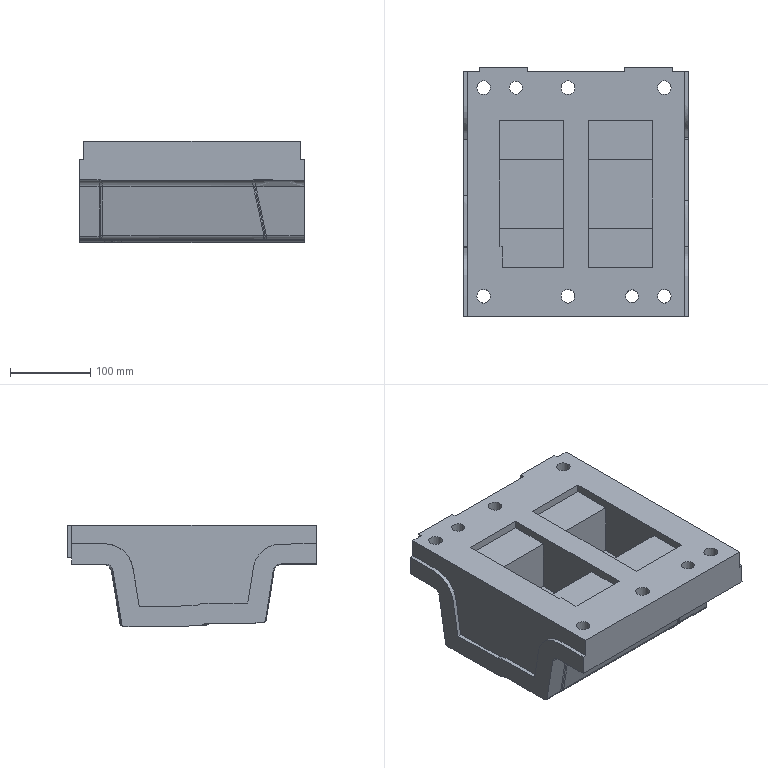Part | NX | features solid 2 | 1 solid | 171 faces | box 280 x 310 x 126.004 mm | volume 6755474 mm3 | plane 66 | spline 62 | cylinder 41 | cone 1 | sphere 1 | commonest cylinder face diameters 10 x7 8 x6 12 x6 17 x6 26 x6 20 x5